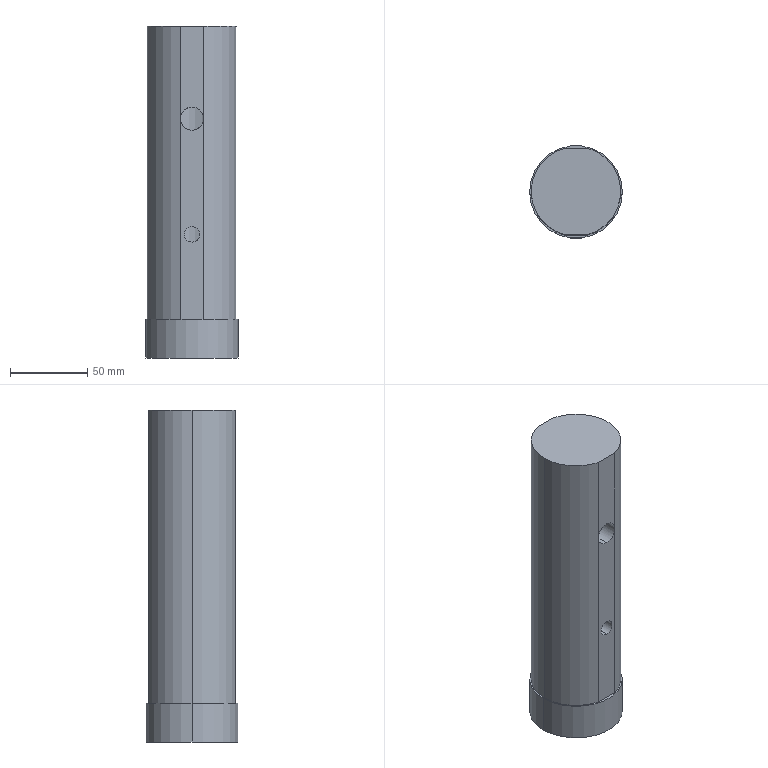Part | SolidWorks | features ICE 6, Chamfer 1, Extrusion 1 | 1 solid | 25 faces | box 60 x 60 x 215 mm | volume 337627 mm3 | cylinder 15 | plane 8 | cone 2 | commonest cylinder face diameters 58 x3 10 x2 15 x2 36 x2 48 x2 48.2 x2
STEP:
#1=CARTESIAN_POINT('',(24.,0.,-24.));
#2=VERTEX_POINT('',#1);
#3=CARTESIAN_POINT('',(-24.,0.,-24.));
#4=VERTEX_POINT('',#3);
#5=CARTESIAN_POINT('',(0.,0.,-24.));
#6=DIRECTION('',(0.,0.,-1.));
#7=DIRECTION('',(-1.,0.,0.));
#8=AXIS2_PLACEMENT_3D('',#5,#6,#7);
#9=CIRCLE('',#8,24.);
#10=EDGE_CURVE('',#2,#4,#9,.T.);
#11=ORIENTED_EDGE('',*,*,#10,.F.);
#12=CARTESIAN_POINT('',(25.,0.,-25.));
#13=VERTEX_POINT('',#12);
#14=CARTESIAN_POINT('',(24.,0.,-24.));
#15=DIRECTION('',(0.7071,0.,-0.7071));
#16=VECTOR('',#15,1000.);
#17=LINE('',#14,#16);
#18=EDGE_CURVE('',#2,#13,#17,.T.);
#19=ORIENTED_EDGE('',*,*,#18,.T.);
#20=CARTESIAN_POINT('',(-25.,0.,-25.));
#21=VERTEX_POINT('',#20);
#22=CARTESIAN_POINT('',(0.,0.,-25.));
#23=DIRECTION('',(0.,0.,1.));
#24=DIRECTION('',(-1.,0.,0.));
#25=AXIS2_PLACEMENT_3D('',#22,#23,#24);
#26=CIRCLE('',#25,25.);
#27=EDGE_CURVE('',#21,#13,#26,.T.);
#28=ORIENTED_EDGE('',*,*,#27,.F.);
#29=CARTESIAN_POINT('',(-24.,0.,-24.));
#30=DIRECTION('',(-0.7071,0.,-0.7071));
#31=VECTOR('',#30,1000.);
#32=LINE('',#29,#31);
#33=EDGE_CURVE('',#4,#21,#32,.T.);
#34=ORIENTED_EDGE('',*,*,#33,.F.);
#35=EDGE_LOOP('',(#11,#19,#28,#34));
#36=FACE_OUTER_BOUND('',#35,.T.);
#37=CARTESIAN_POINT('',(0.,0.,-24.));
#38=DIRECTION('',(0.,0.,-1.));
#39=DIRECTION('',(-1.,0.,0.));
#40=AXIS2_PLACEMENT_3D('',#37,#38,#39);
#41=CONICAL_SURFACE('',#40,24.,0.7854);
#42=ADVANCED_FACE('',(#36),#41,.F.);
#43=CARTESIAN_POINT('',(0.,-28.,60.));
#44=VERTEX_POINT('',#43);
#45=CARTESIAN_POINT('',(0.,-28.,50.));
#46=VERTEX_POINT('',#45);
#47=CARTESIAN_POINT('',(0.,-28.,55.));
#48=DIRECTION('',(0.,-1.,0.));
#49=DIRECTION('',(1.,0.,0.));
#50=AXIS2_PLACEMENT_3D('',#47,#48,#49);
#51=CIRCLE('',#50,5.);
#52=EDGE_CURVE('',#44,#46,#51,.T.);
#53=ORIENTED_EDGE('',*,*,#52,.T.);
#54=CARTESIAN_POINT('',(0.,-18.,50.));
#55=VERTEX_POINT('',#54);
#56=CARTESIAN_POINT('',(0.,-180.,50.));
#57=DIRECTION('',(0.,1.,0.));
#58=VECTOR('',#57,1000.);
#59=LINE('',#56,#58);
#60=EDGE_CURVE('',#46,#55,#59,.T.);
#61=ORIENTED_EDGE('',*,*,#60,.T.);
#62=CARTESIAN_POINT('',(0.,-18.,60.));
#63=VERTEX_POINT('',#62);
#64=CARTESIAN_POINT('',(0.,-18.,60.));
#65=CARTESIAN_POINT('',(-0.3321,-18.,60.));
#66=CARTESIAN_POINT('',(-0.6584,-17.991,59.967));
#67=CARTESIAN_POINT('',(-1.3,-17.956,59.839));
#68=CARTESIAN_POINT('',(-1.618,-17.93,59.742));
#69=CARTESIAN_POINT('',(-2.223,-17.865,59.491));
#70=CARTESIAN_POINT('',(-2.51,-17.826,59.337));
#71=CARTESIAN_POINT('',(-3.052,-17.741,58.974));
#72=CARTESIAN_POINT('',(-3.307,-17.695,58.764));
#73=CARTESIAN_POINT('',(-3.766,-17.603,58.305));
#74=CARTESIAN_POINT('',(-3.972,-17.557,58.054));
#75=CARTESIAN_POINT('',(-4.338,-17.47,57.508));
#76=CARTESIAN_POINT('',(-4.492,-17.431,57.22));
#77=CARTESIAN_POINT('',(-4.679,-17.381,56.769));
#78=CARTESIAN_POINT('',(-4.735,-17.366,56.615));
#79=CARTESIAN_POINT('',(-4.83,-17.34,56.302));
#80=CARTESIAN_POINT('',(-4.871,-17.328,56.14));
#81=CARTESIAN_POINT('',(-4.968,-17.301,55.656));
#82=CARTESIAN_POINT('',(-5.,-17.292,55.33));
#83=CARTESIAN_POINT('',(-5.,-17.292,54.674));
#84=CARTESIAN_POINT('',(-4.967,-17.301,54.341));
#85=CARTESIAN_POINT('',(-4.839,-17.338,53.698));
#86=CARTESIAN_POINT('',(-4.744,-17.364,53.386));
#87=CARTESIAN_POINT('',(-4.491,-17.431,52.778));
#88=CARTESIAN_POINT('',(-4.336,-17.471,52.489));
#89=CARTESIAN_POINT('',(-3.974,-17.557,51.949));
#90=CARTESIAN_POINT('',(-3.766,-17.603,51.695));
#91=CARTESIAN_POINT('',(-3.303,-17.696,51.232));
#92=CARTESIAN_POINT('',(-3.053,-17.741,51.027));
#93=CARTESIAN_POINT('',(-2.512,-17.826,50.665));
#94=CARTESIAN_POINT('',(-2.219,-17.865,50.508));
#95=CARTESIAN_POINT('',(-1.616,-17.93,50.257));
#96=CARTESIAN_POINT('',(-1.304,-17.956,50.162));
#97=CARTESIAN_POINT('',(-0.8205,-17.982,50.065));
#98=CARTESIAN_POINT('',(-0.6557,-17.989,50.04));
#99=CARTESIAN_POINT('',(-0.3275,-17.998,50.008));
#100=CARTESIAN_POINT('',(-0.1637,-18.,50.));
#101=CARTESIAN_POINT('',(0.,-18.,50.));
#102=B_SPLINE_CURVE_WITH_KNOTS('',3,(#64,#65,#66,#67,#68,#69,#70,#71,#72,#73,#74,#75,#76,#77,#78,#79,#80,#81,#82,#83,#84,#85,#86,#87,#88,#89,#90,#91,#92,#93,#94,#95,#96,#97,#98,#99,#100,#101),.UNSPECIFIED.,.F.,.F.,(4,2,2,2,2,2,2,2,2,2,2,2,2,2,2,2,2,2,4),(0.,0.0009819,0.001964,0.002946,0.003927,0.004909,0.005891,0.006382,0.006873,0.007855,0.008837,0.009819,0.0108,0.01178,0.01276,0.01375,0.01473,0.01522,0.01571),.UNSPECIFIED.);
#103=EDGE_CURVE('',#63,#55,#102,.T.);
#104=ORIENTED_EDGE('',*,*,#103,.F.);
#105=CARTESIAN_POINT('',(0.,-180.,60.));
#106=DIRECTION('',(0.,1.,0.));
#107=VECTOR('',#106,1000.);
#108=LINE('',#105,#107);
#109=EDGE_CURVE('',#44,#63,#108,.T.);
#110=ORIENTED_EDGE('',*,*,#109,.F.);
#111=EDGE_LOOP('',(#53,#61,#104,#110));
#112=FACE_OUTER_BOUND('',#111,.T.);
#113=CARTESIAN_POINT('',(0.,-180.,55.));
#114=DIRECTION('',(0.,1.,0.));
#115=DIRECTION('',(0.,0.,1.));
#116=AXIS2_PLACEMENT_3D('',#113,#114,#115);
#117=CYLINDRICAL_SURFACE('',#116,5.);
#118=ADVANCED_FACE('',(#112),#117,.F.);
#119=CARTESIAN_POINT('',(0.,-28.,137.5));
#120=VERTEX_POINT('',#119);
#121=CARTESIAN_POINT('',(0.,-28.,122.5));
#122=VERTEX_POINT('',#121);
#123=CARTESIAN_POINT('',(0.,-28.,130.));
#124=DIRECTION('',(0.,-1.,0.));
#125=DIRECTION('',(1.,0.,0.));
#126=AXIS2_PLACEMENT_3D('',#123,#124,#125);
#127=CIRCLE('',#126,7.5);
#128=EDGE_CURVE('',#120,#122,#127,.T.);
#129=ORIENTED_EDGE('',*,*,#128,.T.);
#130=CARTESIAN_POINT('',(0.,-18.,122.5));
#131=VERTEX_POINT('',#130);
#132=CARTESIAN_POINT('',(0.,-180.,122.5));
#133=DIRECTION('',(0.,1.,0.));
#134=VECTOR('',#133,1000.);
#135=LINE('',#132,#134);
#136=EDGE_CURVE('',#122,#131,#135,.T.);
#137=ORIENTED_EDGE('',*,*,#136,.T.);
#138=CARTESIAN_POINT('',(0.,-18.,137.5));
#139=VERTEX_POINT('',#138);
#140=CARTESIAN_POINT('',(0.,-18.,137.5));
#141=CARTESIAN_POINT('',(-0.5017,-18.,137.5));
#142=CARTESIAN_POINT('',(-0.994,-17.979,137.45));
#143=CARTESIAN_POINT('',(-1.719,-17.919,137.305));
#144=CARTESIAN_POINT('',(-1.958,-17.895,137.244));
#145=CARTESIAN_POINT('',(-2.433,-17.836,137.099));
#146=CARTESIAN_POINT('',(-2.667,-17.803,137.014));
#147=CARTESIAN_POINT('',(-3.346,-17.692,136.73));
#148=CARTESIAN_POINT('',(-3.775,-17.605,136.499));
#149=CARTESIAN_POINT('',(-4.384,-17.459,136.09));
#150=CARTESIAN_POINT('',(-4.581,-17.408,135.943));
#151=CARTESIAN_POINT('',(-4.957,-17.305,135.634));
#152=CARTESIAN_POINT('',(-5.136,-17.253,135.471));
#153=CARTESIAN_POINT('',(-5.649,-17.094,134.958));
#154=CARTESIAN_POINT('',(-5.958,-16.988,134.582));
#155=CARTESIAN_POINT('',(-6.503,-16.787,133.768));
#156=CARTESIAN_POINT('',(-6.733,-16.695,133.34));
#157=CARTESIAN_POINT('',(-7.015,-16.577,132.665));
#158=CARTESIAN_POINT('',(-7.098,-16.542,132.434));
#159=CARTESIAN_POINT('',(-7.243,-16.479,131.962));
#160=CARTESIAN_POINT('',(-7.305,-16.451,131.719));
#161=CARTESIAN_POINT('',(-7.451,-16.386,130.991));
#162=CARTESIAN_POINT('',(-7.5,-16.363,130.501));
#163=CARTESIAN_POINT('',(-7.5,-16.363,129.757));
#164=CARTESIAN_POINT('',(-7.488,-16.369,129.506));
#165=CARTESIAN_POINT('',(-7.438,-16.391,129.009));
#166=CARTESIAN_POINT('',(-7.402,-16.408,128.764));
#167=CARTESIAN_POINT('',(-7.256,-16.473,128.039));
#168=CARTESIAN_POINT('',(-7.112,-16.537,127.567));
#169=CARTESIAN_POINT('',(-6.73,-16.696,126.654));
#170=CARTESIAN_POINT('',(-6.499,-16.788,126.225));
#171=CARTESIAN_POINT('',(-5.958,-16.988,125.418));
#172=CARTESIAN_POINT('',(-5.644,-17.096,125.038));
#173=CARTESIAN_POINT('',(-4.959,-17.307,124.352));
#174=CARTESIAN_POINT('',(-4.585,-17.411,124.045));
#175=CARTESIAN_POINT('',(-3.977,-17.556,123.637));
#176=CARTESIAN_POINT('',(-3.766,-17.603,123.509));
#177=CARTESIAN_POINT('',(-3.334,-17.69,123.277));
#178=CARTESIAN_POINT('',(-3.113,-17.73,123.172));
#179=CARTESIAN_POINT('',(-2.437,-17.84,122.89));
#180=CARTESIAN_POINT('',(-1.968,-17.899,122.746));
#181=CARTESIAN_POINT('',(-0.9885,-17.98,122.549));
#182=CARTESIAN_POINT('',(-0.4942,-18.,122.5));
#183=CARTESIAN_POINT('',(0.,-18.,122.5));
#184=B_SPLINE_CURVE_WITH_KNOTS('',3,(#140,#141,#142,#143,#144,#145,#146,#147,#148,#149,#150,#151,#152,#153,#154,#155,#156,#157,#158,#159,#160,#161,#162,#163,#164,#165,#166,#167,#168,#169,#170,#171,#172,#173,#174,#175,#176,#177,#178,#179,#180,#181,#182,#183),.UNSPECIFIED.,.F.,.F.,(4,2,2,2,2,2,2,2,2,2,2,2,2,2,2,2,2,2,2,2,2,4),(0.,0.001483,0.002224,0.002965,0.004448,0.005189,0.005931,0.007413,0.008896,0.009637,0.01038,0.01186,0.0126,0.01334,0.01483,0.01631,0.01779,0.01927,0.02002,0.02076,0.02224,0.02372),.UNSPECIFIED.);
#185=EDGE_CURVE('',#139,#131,#184,.T.);
#186=ORIENTED_EDGE('',*,*,#185,.F.);
#187=CARTESIAN_POINT('',(0.,-180.,137.5));
#188=DIRECTION('',(0.,1.,0.));
#189=VECTOR('',#188,1000.);
#190=LINE('',#187,#189);
#191=EDGE_CURVE('',#120,#139,#190,.T.);
#192=ORIENTED_EDGE('',*,*,#191,.F.);
#193=EDGE_LOOP('',(#129,#137,#186,#192));
#194=FACE_OUTER_BOUND('',#193,.T.);
#195=CARTESIAN_POINT('',(0.,-180.,130.));
#196=DIRECTION('',(0.,1.,0.));
#197=DIRECTION('',(0.,0.,1.));
#198=AXIS2_PLACEMENT_3D('',#195,#196,#197);
#199=CYLINDRICAL_SURFACE('',#198,7.5);
#200=ADVANCED_FACE('',(#194),#199,.F.);
#201=ORIENTED_EDGE('',*,*,#103,.T.);
#202=CARTESIAN_POINT('',(0.,-18.,50.));
#203=CARTESIAN_POINT('',(0.3272,-18.,50.));
#204=CARTESIAN_POINT('',(0.6546,-17.991,50.032));
#205=CARTESIAN_POINT('',(1.304,-17.956,50.162));
#206=CARTESIAN_POINT('',(1.617,-17.93,50.257));
#207=CARTESIAN_POINT('',(2.219,-17.865,50.508));
#208=CARTESIAN_POINT('',(2.512,-17.826,50.664));
#209=CARTESIAN_POINT('',(3.053,-17.741,51.027));
#210=CARTESIAN_POINT('',(3.304,-17.696,51.233));
#211=CARTESIAN_POINT('',(3.765,-17.603,51.694));
#212=CARTESIAN_POINT('',(3.975,-17.557,51.949));
#213=CARTESIAN_POINT('',(4.336,-17.471,52.489));
#214=CARTESIAN_POINT('',(4.49,-17.432,52.775));
#215=CARTESIAN_POINT('',(4.743,-17.364,53.384));
#216=CARTESIAN_POINT('',(4.838,-17.338,53.698));
#217=CARTESIAN_POINT('',(4.935,-17.31,54.178));
#218=CARTESIAN_POINT('',(4.959,-17.303,54.34));
#219=CARTESIAN_POINT('',(4.992,-17.294,54.668));
#220=CARTESIAN_POINT('',(5.,-17.292,54.834));
#221=CARTESIAN_POINT('',(5.,-17.292,55.329));
#222=CARTESIAN_POINT('',(4.968,-17.301,55.654));
#223=CARTESIAN_POINT('',(4.84,-17.337,56.298));
#224=CARTESIAN_POINT('',(4.743,-17.364,56.617));
#225=CARTESIAN_POINT('',(4.492,-17.431,57.219));
#226=CARTESIAN_POINT('',(4.339,-17.47,57.506));
#227=CARTESIAN_POINT('',(3.974,-17.557,58.052));
#228=CARTESIAN_POINT('',(3.766,-17.603,58.304));
#229=CARTESIAN_POINT('',(3.423,-17.672,58.648));
#230=CARTESIAN_POINT('',(3.302,-17.695,58.758));
#231=CARTESIAN_POINT('',(3.05,-17.74,58.965));
#232=CARTESIAN_POINT('',(2.918,-17.762,59.064));
#233=CARTESIAN_POINT('',(2.51,-17.826,59.336));
#234=CARTESIAN_POINT('',(2.224,-17.865,59.49));
#235=CARTESIAN_POINT('',(1.622,-17.929,59.741));
#236=CARTESIAN_POINT('',(1.303,-17.956,59.838));
#237=CARTESIAN_POINT('',(0.6589,-17.991,59.967));
#238=CARTESIAN_POINT('',(0.332,-18.,60.));
#239=CARTESIAN_POINT('',(0.,-18.,60.));
#240=B_SPLINE_CURVE_WITH_KNOTS('',3,(#202,#203,#204,#205,#206,#207,#208,#209,#210,#211,#212,#213,#214,#215,#216,#217,#218,#219,#220,#221,#222,#223,#224,#225,#226,#227,#228,#229,#230,#231,#232,#233,#234,#235,#236,#237,#238,#239),.UNSPECIFIED.,.F.,.F.,(4,2,2,2,2,2,2,2,2,2,2,2,2,2,2,2,2,2,4),(0.01571,0.01669,0.01767,0.01865,0.01964,0.02062,0.0216,0.02258,0.02307,0.02356,0.02454,0.02553,0.02651,0.02749,0.02798,0.02847,0.02945,0.03043,0.03142),.UNSPECIFIED.);
#241=EDGE_CURVE('',#55,#63,#240,.T.);
#242=ORIENTED_EDGE('',*,*,#241,.T.);
#243=EDGE_LOOP('',(#201,#242));
#244=FACE_BOUND('',#243,.T.);
#245=ORIENTED_EDGE('',*,*,#185,.T.);
#246=CARTESIAN_POINT('',(0.,-18.,122.5));
#247=CARTESIAN_POINT('',(0.2469,-18.,122.5));
#248=CARTESIAN_POINT('',(0.4942,-17.995,122.512));
#249=CARTESIAN_POINT('',(0.9895,-17.974,122.561));
#250=CARTESIAN_POINT('',(1.238,-17.959,122.599));
#251=CARTESIAN_POINT('',(1.967,-17.899,122.746));
#252=CARTESIAN_POINT('',(2.436,-17.84,122.89));
#253=CARTESIAN_POINT('',(3.117,-17.729,123.174));
#254=CARTESIAN_POINT('',(3.341,-17.689,123.281));
#255=CARTESIAN_POINT('',(3.773,-17.601,123.514));
#256=CARTESIAN_POINT('',(3.982,-17.555,123.64));
#257=CARTESIAN_POINT('',(4.385,-17.459,123.91));
#258=CARTESIAN_POINT('',(4.579,-17.409,124.055));
#259=CARTESIAN_POINT('',(4.954,-17.306,124.364));
#260=CARTESIAN_POINT('',(5.135,-17.253,124.529));
#261=CARTESIAN_POINT('',(5.653,-17.093,125.047));
#262=CARTESIAN_POINT('',(5.959,-16.987,125.42));
#263=CARTESIAN_POINT('',(6.364,-16.838,126.024));
#264=CARTESIAN_POINT('',(6.49,-16.79,126.232));
#265=CARTESIAN_POINT('',(6.722,-16.698,126.664));
#266=CARTESIAN_POINT('',(6.828,-16.655,126.888));
#267=CARTESIAN_POINT('',(7.111,-16.537,127.565));
#268=CARTESIAN_POINT('',(7.254,-16.474,128.033));
#269=CARTESIAN_POINT('',(7.401,-16.408,128.759));
#270=CARTESIAN_POINT('',(7.438,-16.391,129.006));
#271=CARTESIAN_POINT('',(7.488,-16.369,129.503));
#272=CARTESIAN_POINT('',(7.5,-16.363,129.751));
#273=CARTESIAN_POINT('',(7.5,-16.363,130.492));
#274=CARTESIAN_POINT('',(7.452,-16.385,130.984));
#275=CARTESIAN_POINT('',(7.256,-16.473,131.964));
#276=CARTESIAN_POINT('',(7.111,-16.537,132.434));
#277=CARTESIAN_POINT('',(6.734,-16.694,133.338));
#278=CARTESIAN_POINT('',(6.499,-16.788,133.775));
#279=CARTESIAN_POINT('',(5.957,-16.988,134.582));
#280=CARTESIAN_POINT('',(5.65,-17.094,134.956));
#281=CARTESIAN_POINT('',(5.134,-17.253,135.473));
#282=CARTESIAN_POINT('',(4.952,-17.306,135.638));
#283=CARTESIAN_POINT('',(4.577,-17.41,135.947));
#284=CARTESIAN_POINT('',(4.382,-17.46,136.092));
#285=CARTESIAN_POINT('',(3.779,-17.604,136.497));
#286=CARTESIAN_POINT('',(3.349,-17.692,136.729));
#287=CARTESIAN_POINT('',(2.435,-17.841,137.111));
#288=CARTESIAN_POINT('',(1.965,-17.899,137.255));
#289=CARTESIAN_POINT('',(1.242,-17.959,137.401));
#290=CARTESIAN_POINT('',(0.9974,-17.974,137.438));
#291=CARTESIAN_POINT('',(0.5023,-17.995,137.487));
#292=CARTESIAN_POINT('',(0.2507,-18.,137.5));
#293=CARTESIAN_POINT('',(0.,-18.,137.5));
#294=B_SPLINE_CURVE_WITH_KNOTS('',3,(#246,#247,#248,#249,#250,#251,#252,#253,#254,#255,#256,#257,#258,#259,#260,#261,#262,#263,#264,#265,#266,#267,#268,#269,#270,#271,#272,#273,#274,#275,#276,#277,#278,#279,#280,#281,#282,#283,#284,#285,#286,#287,#288,#289,#290,#291,#292,#293),.UNSPECIFIED.,.F.,.F.,(4,2,2,2,2,2,2,2,2,2,2,2,2,2,2,2,2,2,2,2,2,2,2,4),(0.02372,0.02446,0.0252,0.02669,0.02743,0.02817,0.02891,0.02965,0.03113,0.03187,0.03261,0.03409,0.03483,0.03557,0.03706,0.03854,0.04002,0.0415,0.04224,0.04298,0.04446,0.04594,0.04668,0.04743),.UNSPECIFIED.);
#295=EDGE_CURVE('',#131,#139,#294,.T.);
#296=ORIENTED_EDGE('',*,*,#295,.T.);
#297=EDGE_LOOP('',(#245,#296));
#298=FACE_BOUND('',#297,.T.);
#299=CARTESIAN_POINT('',(18.,0.,180.));
#300=VERTEX_POINT('',#299);
#301=CARTESIAN_POINT('',(-18.,0.,180.));
#302=VERTEX_POINT('',#301);
#303=CARTESIAN_POINT('',(0.,0.,180.));
#304=DIRECTION('',(0.,0.,-1.));
#305=DIRECTION('',(-1.,0.,0.));
#306=AXIS2_PLACEMENT_3D('',#303,#304,#305);
#307=CIRCLE('',#306,18.);
#308=EDGE_CURVE('',#300,#302,#307,.T.);
#309=ORIENTED_EDGE('',*,*,#308,.F.);
#310=CARTESIAN_POINT('',(18.,0.,0.));
#311=VERTEX_POINT('',#310);
#312=CARTESIAN_POINT('',(18.,0.,180.));
#313=DIRECTION('',(0.,0.,-1.));
#314=VECTOR('',#313,1000.);
#315=LINE('',#312,#314);
#316=EDGE_CURVE('',#300,#311,#315,.T.);
#317=ORIENTED_EDGE('',*,*,#316,.T.);
#318=CARTESIAN_POINT('',(-18.,0.,0.));
#319=VERTEX_POINT('',#318);
#320=CARTESIAN_POINT('',(0.,0.,0.));
#321=DIRECTION('',(0.,0.,-1.));
#322=DIRECTION('',(-1.,0.,0.));
#323=AXIS2_PLACEMENT_3D('',#320,#321,#322);
#324=CIRCLE('',#323,18.);
#325=EDGE_CURVE('',#311,#319,#324,.T.);
#326=ORIENTED_EDGE('',*,*,#325,.T.);
#327=CARTESIAN_POINT('',(-18.,0.,180.));
#328=DIRECTION('',(0.,0.,-1.));
#329=VECTOR('',#328,1000.);
#330=LINE('',#327,#329);
#331=EDGE_CURVE('',#302,#319,#330,.T.);
#332=ORIENTED_EDGE('',*,*,#331,.F.);
#333=EDGE_LOOP('',(#309,#317,#326,#332));
#334=FACE_OUTER_BOUND('',#333,.T.);
#335=CARTESIAN_POINT('',(0.,0.,180.));
#336=DIRECTION('',(0.,0.,-1.));
#337=DIRECTION('',(-1.,0.,0.));
#338=AXIS2_PLACEMENT_3D('',#335,#336,#337);
#339=CYLINDRICAL_SURFACE('',#338,18.);
#340=ADVANCED_FACE('',(#244,#298,#334),#339,.F.);
#341=CARTESIAN_POINT('',(24.1,0.,0.));
#342=VERTEX_POINT('',#341);
#343=CARTESIAN_POINT('',(-24.1,0.,0.));
#344=VERTEX_POINT('',#343);
#345=CARTESIAN_POINT('',(0.,0.,0.));
#346=DIRECTION('',(0.,0.,-1.));
#347=DIRECTION('',(-1.,0.,0.));
#348=AXIS2_PLACEMENT_3D('',#345,#346,#347);
#349=CIRCLE('',#348,24.1);
#350=EDGE_CURVE('',#342,#344,#349,.T.);
#351=ORIENTED_EDGE('',*,*,#350,.F.);
#352=CARTESIAN_POINT('',(24.1,0.,-3.));
#353=VERTEX_POINT('',#352);
#354=CARTESIAN_POINT('',(24.1,0.,0.));
#355=DIRECTION('',(0.,0.,-1.));
#356=VECTOR('',#355,1000.);
#357=LINE('',#354,#356);
#358=EDGE_CURVE('',#342,#353,#357,.T.);
#359=ORIENTED_EDGE('',*,*,#358,.T.);
#360=CARTESIAN_POINT('',(-24.1,0.,-3.));
#361=VERTEX_POINT('',#360);
#362=CARTESIAN_POINT('',(0.,0.,-3.));
#363=DIRECTION('',(0.,0.,-1.));
#364=DIRECTION('',(-1.,0.,0.));
#365=AXIS2_PLACEMENT_3D('',#362,#363,#364);
#366=CIRCLE('',#365,24.1);
#367=EDGE_CURVE('',#353,#361,#366,.T.);
#368=ORIENTED_EDGE('',*,*,#367,.T.);
#369=CARTESIAN_POINT('',(-24.1,0.,0.));
#370=DIRECTION('',(0.,0.,-1.));
#371=VECTOR('',#370,1000.);
#372=LINE('',#369,#371);
#373=EDGE_CURVE('',#344,#361,#372,.T.);
#374=ORIENTED_EDGE('',*,*,#373,.F.);
#375=EDGE_LOOP('',(#351,#359,#368,#374));
#376=FACE_OUTER_BOUND('',#375,.T.);
#377=CARTESIAN_POINT('',(0.,0.,0.));
#378=DIRECTION('',(0.,0.,-1.));
#379=DIRECTION('',(-1.,0.,0.));
#380=AXIS2_PLACEMENT_3D('',#377,#378,#379);
#381=CYLINDRICAL_SURFACE('',#380,24.1);
#382=ADVANCED_FACE('',(#376),#381,.F.);
#383=CARTESIAN_POINT('',(24.,0.,-3.));
#384=VERTEX_POINT('',#383);
#385=CARTESIAN_POINT('',(-24.,0.,-3.));
#386=VERTEX_POINT('',#385);
#387=CARTESIAN_POINT('',(0.,0.,-3.));
#388=DIRECTION('',(0.,0.,-1.));
#389=DIRECTION('',(-1.,0.,0.));
#390=AXIS2_PLACEMENT_3D('',#387,#388,#389);
#391=CIRCLE('',#390,24.);
#392=EDGE_CURVE('',#384,#386,#391,.T.);
#393=ORIENTED_EDGE('',*,*,#392,.F.);
#394=CARTESIAN_POINT('',(24.,0.,-3.));
#395=DIRECTION('',(0.,0.,-1.));
#396=VECTOR('',#395,1000.);
#397=LINE('',#394,#396);
#398=EDGE_CURVE('',#384,#2,#397,.T.);
#399=ORIENTED_EDGE('',*,*,#398,.T.);
#400=ORIENTED_EDGE('',*,*,#10,.T.);
#401=CARTESIAN_POINT('',(-24.,0.,-3.));
#402=DIRECTION('',(0.,0.,-1.));
#403=VECTOR('',#402,1000.);
#404=LINE('',#401,#403);
#405=EDGE_CURVE('',#386,#4,#404,.T.);
#406=ORIENTED_EDGE('',*,*,#405,.F.);
#407=EDGE_LOOP('',(#393,#399,#400,#406));
#408=FACE_OUTER_BOUND('',#407,.T.);
#409=CARTESIAN_POINT('',(0.,0.,-3.));
#410=DIRECTION('',(0.,0.,-1.));
#411=DIRECTION('',(-1.,0.,0.));
#412=AXIS2_PLACEMENT_3D('',#409,#410,#411);
#413=CYLINDRICAL_SURFACE('',#412,24.);
#414=ADVANCED_FACE('',(#408),#413,.F.);
#415=CARTESIAN_POINT('',(-30.,0.,-25.));
#416=VERTEX_POINT('',#415);
#417=CARTESIAN_POINT('',(30.,0.,-25.));
#418=VERTEX_POINT('',#417);
#419=CARTESIAN_POINT('',(0.,0.,-25.));
#420=DIRECTION('',(0.,0.,-1.));
#421=DIRECTION('',(-1.,0.,0.));
#422=AXIS2_PLACEMENT_3D('',#419,#420,#421);
#423=CIRCLE('',#422,30.);
#424=EDGE_CURVE('',#416,#418,#423,.T.);
#425=ORIENTED_EDGE('',*,*,#424,.F.);
#426=CARTESIAN_POINT('',(-30.,0.,0.));
#427=VERTEX_POINT('',#426);
#428=CARTESIAN_POINT('',(-30.,0.,-25.));
#429=DIRECTION('',(0.,0.,1.));
#430=VECTOR('',#429,1000.);
#431=LINE('',#428,#430);
#432=EDGE_CURVE('',#416,#427,#431,.T.);
#433=ORIENTED_EDGE('',*,*,#432,.T.);
#434=CARTESIAN_POINT('',(30.,0.,0.));
#435=VERTEX_POINT('',#434);
#436=CARTESIAN_POINT('',(0.,0.,0.));
#437=DIRECTION('',(0.,0.,-1.));
#438=DIRECTION('',(-1.,0.,0.));
#439=AXIS2_PLACEMENT_3D('',#436,#437,#438);
#440=CIRCLE('',#439,30.);
#441=EDGE_CURVE('',#427,#435,#440,.T.);
#442=ORIENTED_EDGE('',*,*,#441,.T.);
#443=CARTESIAN_POINT('',(30.,0.,-25.));
#444=DIRECTION('',(0.,0.,1.));
#445=VECTOR('',#444,1000.);
#446=LINE('',#443,#445);
#447=EDGE_CURVE('',#418,#435,#446,.T.);
#448=ORIENTED_EDGE('',*,*,#447,.F.);
#449=EDGE_LOOP('',(#425,#433,#442,#448));
#450=FACE_OUTER_BOUND('',#449,.T.);
#451=CARTESIAN_POINT('',(0.,0.,-25.));
#452=DIRECTION('',(0.,0.,1.));
#453=DIRECTION('',(1.,0.,0.));
#454=AXIS2_PLACEMENT_3D('',#451,#452,#453);
#455=CYLINDRICAL_SURFACE('',#454,30.);
#456=ADVANCED_FACE('',(#450),#455,.T.);
#457=CARTESIAN_POINT('',(-29.,0.,190.));
#458=VERTEX_POINT('',#457);
#459=CARTESIAN_POINT('',(-7.55,-28.,190.));
#460=VERTEX_POINT('',#459);
#461=CARTESIAN_POINT('',(0.,0.,190.));
#462=DIRECTION('',(0.,0.,1.));
#463=DIRECTION('',(1.,0.,0.));
#464=AXIS2_PLACEMENT_3D('',#461,#462,#463);
#465=CIRCLE('',#464,29.);
#466=EDGE_CURVE('',#458,#460,#465,.T.);
#467=ORIENTED_EDGE('',*,*,#466,.F.);
#468=CARTESIAN_POINT('',(-29.,0.,0.));
#469=VERTEX_POINT('',#468);
#470=CARTESIAN_POINT('',(-29.,0.,190.));
#471=DIRECTION('',(0.,0.,-1.));
#472=VECTOR('',#471,1000.);
#473=LINE('',#470,#472);
#474=EDGE_CURVE('',#458,#469,#473,.T.);
#475=ORIENTED_EDGE('',*,*,#474,.T.);
#476=CARTESIAN_POINT('',(-7.55,-28.,0.));
#477=VERTEX_POINT('',#476);
#478=CARTESIAN_POINT('',(0.,0.,0.));
#479=DIRECTION('',(0.,0.,1.));
#480=DIRECTION('',(1.,0.,0.));
#481=AXIS2_PLACEMENT_3D('',#478,#479,#480);
#482=CIRCLE('',#481,29.);
#483=EDGE_CURVE('',#469,#477,#482,.T.);
#484=ORIENTED_EDGE('',*,*,#483,.T.);
#485=CARTESIAN_POINT('',(-7.55,-28.,190.));
#486=DIRECTION('',(0.,0.,-1.));
#487=VECTOR('',#486,1000.);
#488=LINE('',#485,#487);
#489=EDGE_CURVE('',#460,#477,#488,.T.);
#490=ORIENTED_EDGE('',*,*,#489,.F.);
#491=EDGE_LOOP('',(#467,#475,#484,#490));
#492=FACE_OUTER_BOUND('',#491,.T.);
#493=CARTESIAN_POINT('',(0.,0.,190.));
#494=DIRECTION('',(0.,0.,-1.));
#495=DIRECTION('',(-1.,0.,0.));
#496=AXIS2_PLACEMENT_3D('',#493,#494,#495);
#497=CYLINDRICAL_SURFACE('',#496,29.);
#498=ADVANCED_FACE('',(#492),#497,.T.);
#499=CARTESIAN_POINT('',(7.55,28.,190.));
#500=VERTEX_POINT('',#499);
#501=CARTESIAN_POINT('',(7.55,28.,0.));
#502=VERTEX_POINT('',#501);
#503=CARTESIAN_POINT('',(7.55,28.,190.));
#504=DIRECTION('',(0.,0.,-1.));
#505=VECTOR('',#504,1000.);
#506=LINE('',#503,#505);
#507=EDGE_CURVE('',#500,#502,#506,.T.);
#508=ORIENTED_EDGE('',*,*,#507,.F.);
#509=CARTESIAN_POINT('',(7.55,-28.,190.));
#510=VERTEX_POINT('',#509);
#511=CARTESIAN_POINT('',(0.,0.,190.));
#512=DIRECTION('',(0.,0.,1.));
#513=DIRECTION('',(1.,0.,0.));
#514=AXIS2_PLACEMENT_3D('',#511,#512,#513);
#515=CIRCLE('',#514,29.);
#516=EDGE_CURVE('',#510,#500,#515,.T.);
#517=ORIENTED_EDGE('',*,*,#516,.F.);
#518=CARTESIAN_POINT('',(7.55,-28.,0.));
#519=VERTEX_POINT('',#518);
#520=CARTESIAN_POINT('',(7.55,-28.,190.));
#521=DIRECTION('',(0.,0.,1.));
#522=VECTOR('',#521,1000.);
#523=LINE('',#520,#522);
#524=EDGE_CURVE('',#519,#510,#523,.T.);
#525=ORIENTED_EDGE('',*,*,#524,.F.);
#526=CARTESIAN_POINT('',(0.,0.,0.));
#527=DIRECTION('',(0.,0.,1.));
#528=DIRECTION('',(1.,0.,0.));
#529=AXIS2_PLACEMENT_3D('',#526,#527,#528);
#530=CIRCLE('',#529,29.);
#531=EDGE_CURVE('',#519,#502,#530,.T.);
#532=ORIENTED_EDGE('',*,*,#531,.T.);
#533=EDGE_LOOP('',(#508,#517,#525,#532));
#534=FACE_OUTER_BOUND('',#533,.T.);
#535=CARTESIAN_POINT('',(0.,0.,190.));
#536=DIRECTION('',(0.,0.,-1.));
#537=DIRECTION('',(-1.,0.,0.));
#538=AXIS2_PLACEMENT_3D('',#535,#536,#537);
#539=CYLINDRICAL_SURFACE('',#538,29.);
#540=ADVANCED_FACE('',(#534),#539,.T.);
#541=ORIENTED_EDGE('',*,*,#474,.F.);
#542=CARTESIAN_POINT('',(-7.55,28.,190.));
#543=VERTEX_POINT('',#542);
#544=CARTESIAN_POINT('',(0.,0.,190.));
#545=DIRECTION('',(0.,0.,1.));
#546=DIRECTION('',(1.,0.,0.));
#547=AXIS2_PLACEMENT_3D('',#544,#545,#546);
#548=CIRCLE('',#547,29.);
#549=EDGE_CURVE('',#543,#458,#548,.T.);
#550=ORIENTED_EDGE('',*,*,#549,.F.);
#551=CARTESIAN_POINT('',(-7.55,28.,0.));
#552=VERTEX_POINT('',#551);
#553=CARTESIAN_POINT('',(-7.55,28.,190.));
#554=DIRECTION('',(0.,0.,1.));
#555=VECTOR('',#554,1000.);
#556=LINE('',#553,#555);
#557=EDGE_CURVE('',#552,#543,#556,.T.);
#558=ORIENTED_EDGE('',*,*,#557,.F.);
#559=CARTESIAN_POINT('',(0.,0.,0.));
#560=DIRECTION('',(0.,0.,1.));
#561=DIRECTION('',(1.,0.,0.));
#562=AXIS2_PLACEMENT_3D('',#559,#560,#561);
#563=CIRCLE('',#562,29.);
#564=EDGE_CURVE('',#552,#469,#563,.T.);
#565=ORIENTED_EDGE('',*,*,#564,.T.);
#566=EDGE_LOOP('',(#541,#550,#558,#565));
#567=FACE_OUTER_BOUND('',#566,.T.);
#568=CARTESIAN_POINT('',(0.,0.,190.));
#569=DIRECTION('',(0.,0.,-1.));
#570=DIRECTION('',(-1.,0.,0.));
#571=AXIS2_PLACEMENT_3D('',#568,#569,#570);
#572=CYLINDRICAL_SURFACE('',#571,29.);
#573=ADVANCED_FACE('',(#567),#572,.T.);
#574=ORIENTED_EDGE('',*,*,#516,.T.);
#575=CARTESIAN_POINT('',(42.099,28.,190.));
#576=DIRECTION('',(-1.,0.,0.));
#577=VECTOR('',#576,1000.);
#578=LINE('',#575,#577);
#579=EDGE_CURVE('',#500,#543,#578,.T.);
#580=ORIENTED_EDGE('',*,*,#579,.T.);
#581=ORIENTED_EDGE('',*,*,#549,.T.);
#582=ORIENTED_EDGE('',*,*,#466,.T.);
#583=CARTESIAN_POINT('',(42.099,-28.,190.));
#584=DIRECTION('',(1.,0.,0.));
#585=VECTOR('',#584,1000.);
#586=LINE('',#583,#585);
#587=EDGE_CURVE('',#460,#510,#586,.T.);
#588=ORIENTED_EDGE('',*,*,#587,.T.);
#589=EDGE_LOOP('',(#574,#580,#581,#582,#588));
#590=FACE_OUTER_BOUND('',#589,.T.);
#591=CARTESIAN_POINT('',(0.,0.,190.));
#592=DIRECTION('',(0.,0.,1.));
#593=DIRECTION('',(1.,0.,0.));
#594=AXIS2_PLACEMENT_3D('',#591,#592,#593);
#595=PLANE('',#594);
#596=ADVANCED_FACE('',(#590),#595,.T.);
#597=ORIENTED_EDGE('',*,*,#432,.F.);
#598=CARTESIAN_POINT('',(0.,0.,-25.));
#599=DIRECTION('',(0.,0.,-1.));
#600=DIRECTION('',(-1.,0.,0.));
#601=AXIS2_PLACEMENT_3D('',#598,#599,#600);
#602=CIRCLE('',#601,30.);
#603=EDGE_CURVE('',#418,#416,#602,.T.);
#604=ORIENTED_EDGE('',*,*,#603,.F.);
#605=ORIENTED_EDGE('',*,*,#447,.T.);
#606=CARTESIAN_POINT('',(0.,0.,0.));
#607=DIRECTION('',(0.,0.,-1.));
#608=DIRECTION('',(-1.,0.,0.));
#609=AXIS2_PLACEMENT_3D('',#606,#607,#608);
#610=CIRCLE('',#609,30.);
#611=EDGE_CURVE('',#435,#427,#610,.T.);
#612=ORIENTED_EDGE('',*,*,#611,.T.);
#613=EDGE_LOOP('',(#597,#604,#605,#612));
#614=FACE_OUTER_BOUND('',#613,.T.);
#615=CARTESIAN_POINT('',(0.,0.,-25.));
#616=DIRECTION('',(0.,0.,1.));
#617=DIRECTION('',(1.,0.,0.));
#618=AXIS2_PLACEMENT_3D('',#615,#616,#617);
#619=CYLINDRICAL_SURFACE('',#618,30.);
#620=ADVANCED_FACE('',(#614),#619,.T.);
#621=ORIENTED_EDGE('',*,*,#27,.T.);
#622=CARTESIAN_POINT('',(0.,0.,-25.));
#623=DIRECTION('',(0.,0.,1.));
#624=DIRECTION('',(-1.,0.,0.));
#625=AXIS2_PLACEMENT_3D('',#622,#623,#624);
#626=CIRCLE('',#625,25.);
#627=EDGE_CURVE('',#13,#21,#626,.T.);
#628=ORIENTED_EDGE('',*,*,#627,.T.);
#629=EDGE_LOOP('',(#621,#628));
#630=FACE_BOUND('',#629,.T.);
#631=ORIENTED_EDGE('',*,*,#603,.T.);
#632=ORIENTED_EDGE('',*,*,#424,.T.);
#633=EDGE_LOOP('',(#631,#632));
#634=FACE_OUTER_BOUND('',#633,.T.);
#635=CARTESIAN_POINT('',(0.,0.,-25.));
#636=DIRECTION('',(0.,0.,-1.));
#637=DIRECTION('',(-1.,0.,0.));
#638=AXIS2_PLACEMENT_3D('',#635,#636,#637);
#639=PLANE('',#638);
#640=ADVANCED_FACE('',(#630,#634),#639,.T.);
#641=ORIENTED_EDGE('',*,*,#564,.F.);
#642=CARTESIAN_POINT('',(42.099,28.,0.));
#643=DIRECTION('',(-1.,0.,0.));
#644=VECTOR('',#643,1000.);
#645=LINE('',#642,#644);
#646=EDGE_CURVE('',#502,#552,#645,.T.);
#647=ORIENTED_EDGE('',*,*,#646,.F.);
#648=ORIENTED_EDGE('',*,*,#531,.F.);
#649=CARTESIAN_POINT('',(42.099,-28.,0.));
#650=DIRECTION('',(1.,0.,0.));
#651=VECTOR('',#650,1000.);
#652=LINE('',#649,#651);
#653=EDGE_CURVE('',#477,#519,#652,.T.);
#654=ORIENTED_EDGE('',*,*,#653,.F.);
#655=ORIENTED_EDGE('',*,*,#483,.F.);
#656=EDGE_LOOP('',(#641,#647,#648,#654,#655));
#657=FACE_BOUND('',#656,.T.);
#658=ORIENTED_EDGE('',*,*,#611,.F.);
#659=ORIENTED_EDGE('',*,*,#441,.F.);
#660=EDGE_LOOP('',(#658,#659));
#661=FACE_OUTER_BOUND('',#660,.T.);
#662=CARTESIAN_POINT('',(0.,0.,0.));
#663=DIRECTION('',(0.,0.,-1.));
#664=DIRECTION('',(-1.,0.,0.));
#665=AXIS2_PLACEMENT_3D('',#662,#663,#664);
#666=PLANE('',#665);
#667=ADVANCED_FACE('',(#657,#661),#666,.F.);
#668=ORIENTED_EDGE('',*,*,#52,.F.);
#669=CARTESIAN_POINT('',(0.,-28.,55.));
#670=DIRECTION('',(0.,-1.,0.));
#671=DIRECTION('',(1.,0.,0.));
#672=AXIS2_PLACEMENT_3D('',#669,#670,#671);
#673=CIRCLE('',#672,5.);
#674=EDGE_CURVE('',#46,#44,#673,.T.);
#675=ORIENTED_EDGE('',*,*,#674,.F.);
#676=EDGE_LOOP('',(#668,#675));
#677=FACE_BOUND('',#676,.T.);
#678=ORIENTED_EDGE('',*,*,#128,.F.);
#679=CARTESIAN_POINT('',(0.,-28.,130.));
#680=DIRECTION('',(0.,-1.,0.));
#681=DIRECTION('',(1.,0.,0.));
#682=AXIS2_PLACEMENT_3D('',#679,#680,#681);
#683=CIRCLE('',#682,7.5);
#684=EDGE_CURVE('',#122,#120,#683,.T.);
#685=ORIENTED_EDGE('',*,*,#684,.F.);
#686=EDGE_LOOP('',(#678,#685));
#687=FACE_BOUND('',#686,.T.);
#688=ORIENTED_EDGE('',*,*,#489,.T.);
#689=ORIENTED_EDGE('',*,*,#653,.T.);
#690=ORIENTED_EDGE('',*,*,#524,.T.);
#691=ORIENTED_EDGE('',*,*,#587,.F.);
#692=EDGE_LOOP('',(#688,#689,#690,#691));
#693=FACE_OUTER_BOUND('',#692,.T.);
#694=CARTESIAN_POINT('',(42.099,-28.,-115.01));
#695=DIRECTION('',(0.,-1.,0.));
#696=DIRECTION('',(1.,0.,0.));
#697=AXIS2_PLACEMENT_3D('',#694,#695,#696);
#698=PLANE('',#697);
#699=ADVANCED_FACE('',(#677,#687,#693),#698,.T.);
#700=ORIENTED_EDGE('',*,*,#507,.T.);
#701=ORIENTED_EDGE('',*,*,#646,.T.);
#702=ORIENTED_EDGE('',*,*,#557,.T.);
#703=ORIENTED_EDGE('',*,*,#579,.F.);
#704=EDGE_LOOP('',(#700,#701,#702,#703));
#705=FACE_OUTER_BOUND('',#704,.T.);
#706=CARTESIAN_POINT('',(42.099,28.,-115.01));
#707=DIRECTION('',(0.,1.,0.));
#708=DIRECTION('',(-1.,0.,0.));
#709=AXIS2_PLACEMENT_3D('',#706,#707,#708);
#710=PLANE('',#709);
#711=ADVANCED_FACE('',(#705),#710,.T.);
#712=ORIENTED_EDGE('',*,*,#398,.F.);
#713=CARTESIAN_POINT('',(0.,0.,-3.));
#714=DIRECTION('',(0.,0.,-1.));
#715=DIRECTION('',(-1.,0.,0.));
#716=AXIS2_PLACEMENT_3D('',#713,#714,#715);
#717=CIRCLE('',#716,24.);
#718=EDGE_CURVE('',#386,#384,#717,.T.);
#719=ORIENTED_EDGE('',*,*,#718,.F.);
#720=ORIENTED_EDGE('',*,*,#405,.T.);
#721=CARTESIAN_POINT('',(0.,0.,-24.));
#722=DIRECTION('',(0.,0.,-1.));
#723=DIRECTION('',(-1.,0.,0.));
#724=AXIS2_PLACEMENT_3D('',#721,#722,#723);
#725=CIRCLE('',#724,24.);
#726=EDGE_CURVE('',#4,#2,#725,.T.);
#727=ORIENTED_EDGE('',*,*,#726,.T.);
#728=EDGE_LOOP('',(#712,#719,#720,#727));
#729=FACE_OUTER_BOUND('',#728,.T.);
#730=CARTESIAN_POINT('',(0.,0.,-3.));
#731=DIRECTION('',(0.,0.,-1.));
#732=DIRECTION('',(-1.,0.,0.));
#733=AXIS2_PLACEMENT_3D('',#730,#731,#732);
#734=CYLINDRICAL_SURFACE('',#733,24.);
#735=ADVANCED_FACE('',(#729),#734,.F.);
#736=ORIENTED_EDGE('',*,*,#358,.F.);
#737=CARTESIAN_POINT('',(0.,0.,0.));
#738=DIRECTION('',(0.,0.,-1.));
#739=DIRECTION('',(-1.,0.,0.));
#740=AXIS2_PLACEMENT_3D('',#737,#738,#739);
#741=CIRCLE('',#740,24.1);
#742=EDGE_CURVE('',#344,#342,#741,.T.);
#743=ORIENTED_EDGE('',*,*,#742,.F.);
#744=ORIENTED_EDGE('',*,*,#373,.T.);
#745=CARTESIAN_POINT('',(0.,0.,-3.));
#746=DIRECTION('',(0.,0.,-1.));
#747=DIRECTION('',(-1.,0.,0.));
#748=AXIS2_PLACEMENT_3D('',#745,#746,#747);
#749=CIRCLE('',#748,24.1);
#750=EDGE_CURVE('',#361,#353,#749,.T.);
#751=ORIENTED_EDGE('',*,*,#750,.T.);
#752=EDGE_LOOP('',(#736,#743,#744,#751));
#753=FACE_OUTER_BOUND('',#752,.T.);
#754=CARTESIAN_POINT('',(0.,0.,0.));
#755=DIRECTION('',(0.,0.,-1.));
#756=DIRECTION('',(-1.,0.,0.));
#757=AXIS2_PLACEMENT_3D('',#754,#755,#756);
#758=CYLINDRICAL_SURFACE('',#757,24.1);
#759=ADVANCED_FACE('',(#753),#758,.F.);
#760=CARTESIAN_POINT('',(0.,0.,0.));
#761=DIRECTION('',(0.,0.,-1.));
#762=DIRECTION('',(-1.,0.,0.));
#763=AXIS2_PLACEMENT_3D('',#760,#761,#762);
#764=CIRCLE('',#763,18.);
#765=EDGE_CURVE('',#319,#311,#764,.T.);
#766=ORIENTED_EDGE('',*,*,#765,.F.);
#767=ORIENTED_EDGE('',*,*,#325,.F.);
#768=EDGE_LOOP('',(#766,#767));
#769=FACE_BOUND('',#768,.T.);
#770=ORIENTED_EDGE('',*,*,#742,.T.);
#771=ORIENTED_EDGE('',*,*,#350,.T.);
#772=EDGE_LOOP('',(#770,#771));
#773=FACE_OUTER_BOUND('',#772,.T.);
#774=CARTESIAN_POINT('',(0.,0.,0.));
#775=DIRECTION('',(0.,0.,-1.));
#776=DIRECTION('',(-1.,0.,0.));
#777=AXIS2_PLACEMENT_3D('',#774,#775,#776);
#778=PLANE('',#777);
#779=ADVANCED_FACE('',(#769,#773),#778,.T.);
#780=ORIENTED_EDGE('',*,*,#718,.T.);
#781=ORIENTED_EDGE('',*,*,#392,.T.);
#782=EDGE_LOOP('',(#780,#781));
#783=FACE_BOUND('',#782,.T.);
#784=ORIENTED_EDGE('',*,*,#750,.F.);
#785=ORIENTED_EDGE('',*,*,#367,.F.);
#786=EDGE_LOOP('',(#784,#785));
#787=FACE_OUTER_BOUND('',#786,.T.);
#788=CARTESIAN_POINT('',(0.,0.,-3.));
#789=DIRECTION('',(0.,0.,-1.));
#790=DIRECTION('',(-1.,0.,0.));
#791=AXIS2_PLACEMENT_3D('',#788,#789,#790);
#792=PLANE('',#791);
#793=ADVANCED_FACE('',(#783,#787),#792,.F.);
#794=ORIENTED_EDGE('',*,*,#316,.F.);
#795=CARTESIAN_POINT('',(0.,0.,180.));
#796=DIRECTION('',(0.,0.,-1.));
#797=DIRECTION('',(-1.,0.,0.));
#798=AXIS2_PLACEMENT_3D('',#795,#796,#797);
#799=CIRCLE('',#798,18.);
#800=EDGE_CURVE('',#302,#300,#799,.T.);
#801=ORIENTED_EDGE('',*,*,#800,.F.);
#802=ORIENTED_EDGE('',*,*,#331,.T.);
#803=ORIENTED_EDGE('',*,*,#765,.T.);
#804=EDGE_LOOP('',(#794,#801,#802,#803));
#805=FACE_OUTER_BOUND('',#804,.T.);
#806=CARTESIAN_POINT('',(0.,0.,180.));
#807=DIRECTION('',(0.,0.,-1.));
#808=DIRECTION('',(-1.,0.,0.));
#809=AXIS2_PLACEMENT_3D('',#806,#807,#808);
#810=CYLINDRICAL_SURFACE('',#809,18.);
#811=ADVANCED_FACE('',(#805),#810,.F.);
#812=ORIENTED_EDGE('',*,*,#800,.T.);
#813=ORIENTED_EDGE('',*,*,#308,.T.);
#814=EDGE_LOOP('',(#812,#813));
#815=FACE_OUTER_BOUND('',#814,.T.);
#816=CARTESIAN_POINT('',(0.,0.,180.));
#817=DIRECTION('',(0.,0.,-1.));
#818=DIRECTION('',(-1.,0.,0.));
#819=AXIS2_PLACEMENT_3D('',#816,#817,#818);
#820=PLANE('',#819);
#821=ADVANCED_FACE('',(#815),#820,.T.);
#822=ORIENTED_EDGE('',*,*,#136,.F.);
#823=ORIENTED_EDGE('',*,*,#684,.T.);
#824=ORIENTED_EDGE('',*,*,#191,.T.);
#825=ORIENTED_EDGE('',*,*,#295,.F.);
#826=EDGE_LOOP('',(#822,#823,#824,#825));
#827=FACE_OUTER_BOUND('',#826,.T.);
#828=CARTESIAN_POINT('',(0.,-180.,130.));
#829=DIRECTION('',(0.,1.,0.));
#830=DIRECTION('',(0.,0.,1.));
#831=AXIS2_PLACEMENT_3D('',#828,#829,#830);
#832=CYLINDRICAL_SURFACE('',#831,7.5);
#833=ADVANCED_FACE('',(#827),#832,.F.);
#834=ORIENTED_EDGE('',*,*,#60,.F.);
#835=ORIENTED_EDGE('',*,*,#674,.T.);
#836=ORIENTED_EDGE('',*,*,#109,.T.);
#837=ORIENTED_EDGE('',*,*,#241,.F.);
#838=EDGE_LOOP('',(#834,#835,#836,#837));
#839=FACE_OUTER_BOUND('',#838,.T.);
#840=CARTESIAN_POINT('',(0.,-180.,55.));
#841=DIRECTION('',(0.,1.,0.));
#842=DIRECTION('',(0.,0.,1.));
#843=AXIS2_PLACEMENT_3D('',#840,#841,#842);
#844=CYLINDRICAL_SURFACE('',#843,5.);
#845=ADVANCED_FACE('',(#839),#844,.F.);
#846=ORIENTED_EDGE('',*,*,#18,.F.);
#847=ORIENTED_EDGE('',*,*,#726,.F.);
#848=ORIENTED_EDGE('',*,*,#33,.T.);
#849=ORIENTED_EDGE('',*,*,#627,.F.);
#850=EDGE_LOOP('',(#846,#847,#848,#849));
#851=FACE_OUTER_BOUND('',#850,.T.);
#852=CARTESIAN_POINT('',(0.,0.,-24.));
#853=DIRECTION('',(0.,0.,-1.));
#854=DIRECTION('',(-1.,0.,0.));
#855=AXIS2_PLACEMENT_3D('',#852,#853,#854);
#856=CONICAL_SURFACE('',#855,24.,0.7854);
#857=ADVANCED_FACE('',(#851),#856,.F.);
#858=CLOSED_SHELL('',(#42,#118,#200,#340,#382,#414,#456,#498,#540,#573,#596,#620,#640,#667,#699,#711,#735,#759,#779,#793,#811,#821,#833,#845,#857));
#859=MANIFOLD_SOLID_BREP('',#858);
#860=CARTESIAN_POINT('',(0.,0.,0.));
#861=DIRECTION('',(0.,0.,1.));
#862=DIRECTION('',(1.,0.,0.));
#863=AXIS2_PLACEMENT_3D('',#860,#861,#862);
#864=(LENGTH_UNIT()NAMED_UNIT(*)SI_UNIT(.MILLI.,.METRE.));
#865=UNCERTAINTY_MEASURE_WITH_UNIT(LENGTH_MEASURE(0.00001),#864,'','');
#866=(NAMED_UNIT(*)PLANE_ANGLE_UNIT()SI_UNIT($,.RADIAN.));
#867=(NAMED_UNIT(*)SI_UNIT($,.STERADIAN.)SOLID_ANGLE_UNIT());
#868=(GEOMETRIC_REPRESENTATION_CONTEXT(3)GLOBAL_UNCERTAINTY_ASSIGNED_CONTEXT((#865))GLOBAL_UNIT_ASSIGNED_CONTEXT((#864,#866,#867))REPRESENTATION_CONTEXT('',''));
#869=ADVANCED_BREP_SHAPE_REPRESENTATION('',(#859,#863),#868);